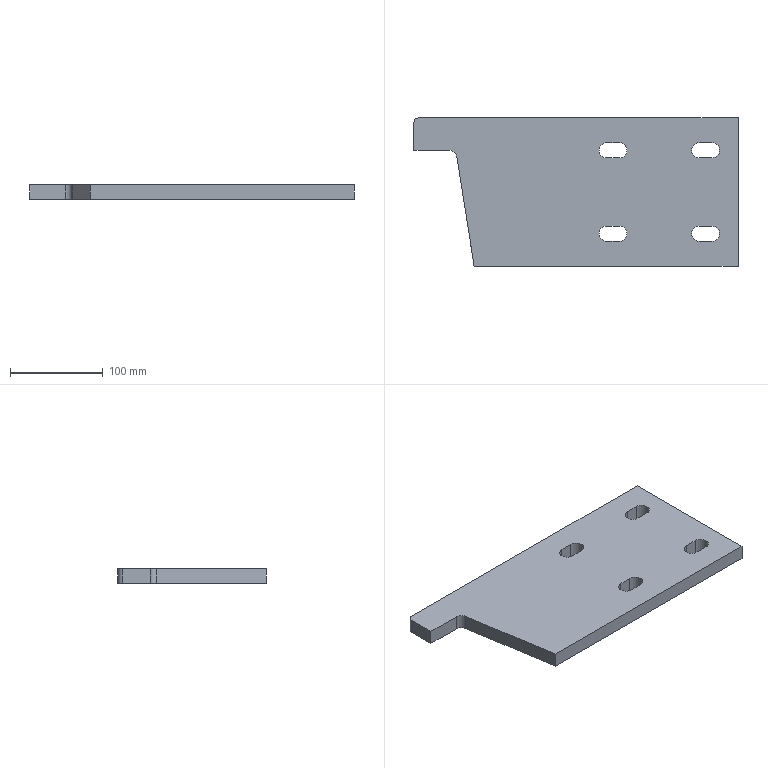Part | STEP file | 03-Connecting plate 1 | 1 solid | 30 faces | box 350 x 160 x 16 mm | volume 757922 mm3 | plane 16 | cylinder 14 | commonest cylinder face diameters 16.5 x12 10 x1 16 x1